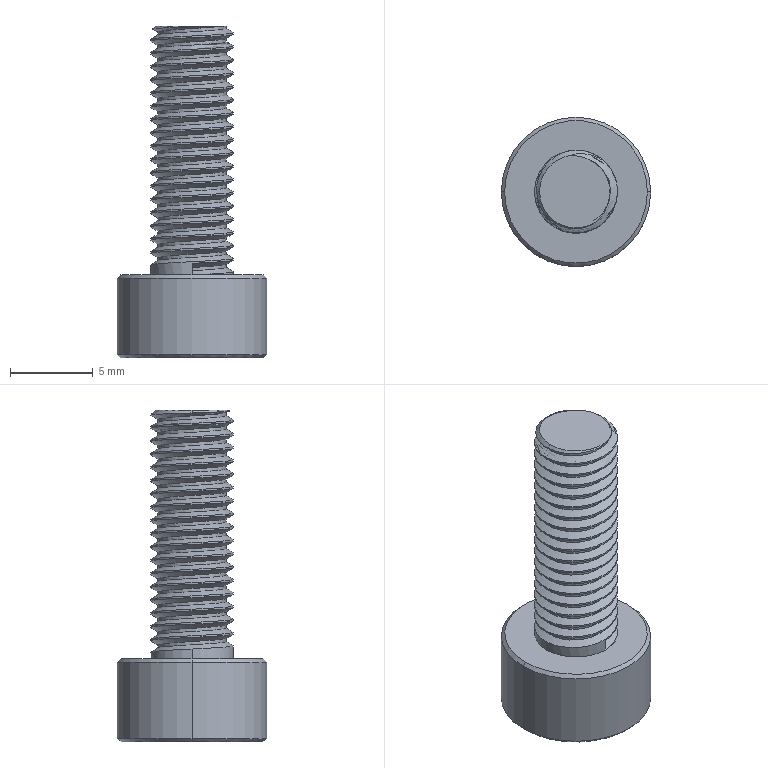Part | 1 solid | 67 faces | box 9 x 9 x 20 mm | volume 529.658 mm3 | cylinder 40 | cone 13 | plane 11 | spline 3 | commonest cylinder face diameters 5 x38 9 x2